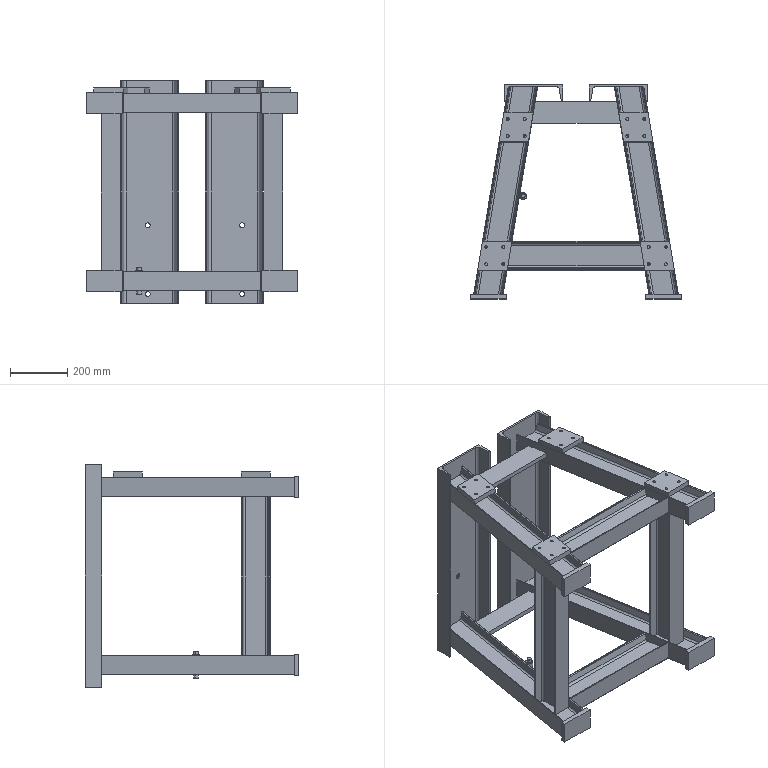Part | SolidWorks | 21 solids | 326 faces | box 738.903 x 747.997 x 780 mm | volume 12463508 mm3 | plane 200 | cylinder 118 | cone 8 | commonest cylinder face diameters 5.6 x32 10.106 x32 14.8 x32 17 x8 6.6 x4 17.8 x4